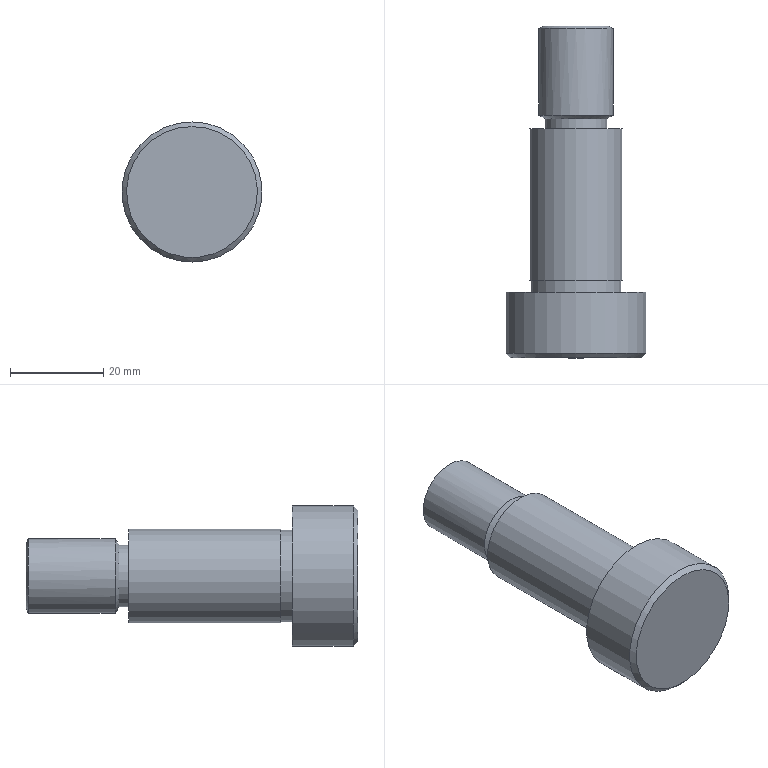Part | STEP file | SCREW-4_id658_x_t | 1 solid | 13 faces | box 30 x 71 x 30 mm | volume 25054 mm3 | plane 5 | cylinder 5 | cone 3 | commonest cylinder face diameters 13.2 x1 16 x1 19.5 x1 20 x1 30 x1
STEP:
#1=CARTESIAN_POINT('',(-162.,76.5,124.));
#2=VERTEX_POINT('',#1);
#3=CARTESIAN_POINT('',(-162.,76.5,110.));
#4=DIRECTION('',(0.,1.,0.));
#5=DIRECTION('',(0.,0.,1.));
#6=AXIS2_PLACEMENT_3D('',#3,#4,#5);
#7=CIRCLE('',#6,14.);
#8=EDGE_CURVE('',#2,#2,#7,.T.);
#9=ORIENTED_EDGE('',*,*,#8,.F.);
#10=EDGE_LOOP('',(#9));
#11=FACE_OUTER_BOUND('',#10,.T.);
#12=CARTESIAN_POINT('',(-162.,76.5,110.));
#13=DIRECTION('',(0.,-1.,0.));
#14=DIRECTION('',(0.,0.,-1.));
#15=AXIS2_PLACEMENT_3D('',#12,#13,#14);
#16=PLANE('',#15);
#17=ADVANCED_FACE('',(#11),#16,.T.);
#18=CARTESIAN_POINT('',(-162.,147.5,103.));
#19=VERTEX_POINT('',#18);
#20=CARTESIAN_POINT('',(-162.,147.5,110.));
#21=DIRECTION('',(0.,-1.,0.));
#22=DIRECTION('',(0.,0.,-1.));
#23=AXIS2_PLACEMENT_3D('',#20,#21,#22);
#24=CIRCLE('',#23,7.);
#25=EDGE_CURVE('',#19,#19,#24,.T.);
#26=ORIENTED_EDGE('',*,*,#25,.F.);
#27=EDGE_LOOP('',(#26));
#28=FACE_OUTER_BOUND('',#27,.T.);
#29=CARTESIAN_POINT('',(-162.,147.5,110.));
#30=DIRECTION('',(0.,-1.,0.));
#31=DIRECTION('',(0.,0.,-1.));
#32=AXIS2_PLACEMENT_3D('',#29,#30,#31);
#33=PLANE('',#32);
#34=ADVANCED_FACE('',(#28),#33,.F.);
#35=ORIENTED_EDGE('',*,*,#8,.T.);
#36=EDGE_LOOP('',(#35));
#37=FACE_BOUND('',#36,.T.);
#38=CARTESIAN_POINT('',(-162.,77.5,95.));
#39=VERTEX_POINT('',#38);
#40=CARTESIAN_POINT('',(-162.,77.5,110.));
#41=DIRECTION('',(0.,1.,0.));
#42=DIRECTION('',(0.,0.,-1.));
#43=AXIS2_PLACEMENT_3D('',#40,#41,#42);
#44=CIRCLE('',#43,15.);
#45=EDGE_CURVE('',#39,#39,#44,.T.);
#46=ORIENTED_EDGE('',*,*,#45,.F.);
#47=EDGE_LOOP('',(#46));
#48=FACE_BOUND('',#47,.T.);
#49=CARTESIAN_POINT('',(-162.,77.5,110.));
#50=DIRECTION('',(0.,1.,0.));
#51=DIRECTION('',(0.,0.,1.));
#52=AXIS2_PLACEMENT_3D('',#49,#50,#51);
#53=CONICAL_SURFACE('',#52,15.,45.);
#54=ADVANCED_FACE('',(#37,#48),#53,.T.);
#55=ORIENTED_EDGE('',*,*,#25,.T.);
#56=EDGE_LOOP('',(#55));
#57=FACE_BOUND('',#56,.T.);
#58=CARTESIAN_POINT('',(-162.,147.,102.));
#59=VERTEX_POINT('',#58);
#60=CARTESIAN_POINT('',(-162.,147.,110.));
#61=DIRECTION('',(0.,-1.,0.));
#62=DIRECTION('',(0.,0.,-1.));
#63=AXIS2_PLACEMENT_3D('',#60,#61,#62);
#64=CIRCLE('',#63,8.);
#65=EDGE_CURVE('',#59,#59,#64,.T.);
#66=ORIENTED_EDGE('',*,*,#65,.F.);
#67=EDGE_LOOP('',(#66));
#68=FACE_BOUND('',#67,.T.);
#69=CARTESIAN_POINT('',(-162.,147.,110.));
#70=DIRECTION('',(0.,-1.,0.));
#71=DIRECTION('',(0.,0.,-1.));
#72=AXIS2_PLACEMENT_3D('',#69,#70,#71);
#73=CONICAL_SURFACE('',#72,8.,63.435);
#74=ADVANCED_FACE('',(#57,#68),#73,.T.);
#75=ORIENTED_EDGE('',*,*,#45,.T.);
#76=EDGE_LOOP('',(#75));
#77=FACE_BOUND('',#76,.T.);
#78=CARTESIAN_POINT('',(-162.,90.5,95.));
#79=VERTEX_POINT('',#78);
#80=CARTESIAN_POINT('',(-162.,90.5,110.));
#81=DIRECTION('',(0.,-1.,0.));
#82=DIRECTION('',(0.,0.,-1.));
#83=AXIS2_PLACEMENT_3D('',#80,#81,#82);
#84=CIRCLE('',#83,15.);
#85=EDGE_CURVE('',#79,#79,#84,.T.);
#86=ORIENTED_EDGE('',*,*,#85,.T.);
#87=EDGE_LOOP('',(#86));
#88=FACE_BOUND('',#87,.T.);
#89=CARTESIAN_POINT('',(-162.,72.95,110.));
#90=DIRECTION('',(0.,-1.,0.));
#91=DIRECTION('',(0.,0.,-1.));
#92=AXIS2_PLACEMENT_3D('',#89,#90,#91);
#93=CYLINDRICAL_SURFACE('',#92,15.);
#94=ADVANCED_FACE('',(#77,#88),#93,.T.);
#95=ORIENTED_EDGE('',*,*,#65,.T.);
#96=EDGE_LOOP('',(#95));
#97=FACE_BOUND('',#96,.T.);
#98=CARTESIAN_POINT('',(-154.,128.45,110.));
#99=VERTEX_POINT('',#98);
#100=CARTESIAN_POINT('',(-162.,128.45,110.));
#101=DIRECTION('',(0.,-1.,0.));
#102=DIRECTION('',(1.,0.,0.));
#103=AXIS2_PLACEMENT_3D('',#100,#101,#102);
#104=CIRCLE('',#103,8.);
#105=EDGE_CURVE('',#99,#99,#104,.T.);
#106=ORIENTED_EDGE('',*,*,#105,.F.);
#107=EDGE_LOOP('',(#106));
#108=FACE_BOUND('',#107,.T.);
#109=CARTESIAN_POINT('',(-162.,72.95,110.));
#110=DIRECTION('',(0.,-1.,0.));
#111=DIRECTION('',(0.,0.,-1.));
#112=AXIS2_PLACEMENT_3D('',#109,#110,#111);
#113=CYLINDRICAL_SURFACE('',#112,8.);
#114=ADVANCED_FACE('',(#97,#108),#113,.T.);
#115=CARTESIAN_POINT('',(-162.,90.5,100.25));
#116=VERTEX_POINT('',#115);
#117=CARTESIAN_POINT('',(-162.,90.5,110.));
#118=DIRECTION('',(0.,1.,0.));
#119=DIRECTION('',(0.,0.,-1.));
#120=AXIS2_PLACEMENT_3D('',#117,#118,#119);
#121=CIRCLE('',#120,9.75);
#122=EDGE_CURVE('',#116,#116,#121,.T.);
#123=ORIENTED_EDGE('',*,*,#122,.F.);
#124=EDGE_LOOP('',(#123));
#125=FACE_BOUND('',#124,.T.);
#126=ORIENTED_EDGE('',*,*,#85,.F.);
#127=EDGE_LOOP('',(#126));
#128=FACE_BOUND('',#127,.T.);
#129=CARTESIAN_POINT('',(-162.,90.5,110.));
#130=DIRECTION('',(0.,-1.,0.));
#131=DIRECTION('',(0.,0.,-1.));
#132=AXIS2_PLACEMENT_3D('',#129,#130,#131);
#133=PLANE('',#132);
#134=ADVANCED_FACE('',(#125,#128),#133,.F.);
#135=ORIENTED_EDGE('',*,*,#105,.T.);
#136=EDGE_LOOP('',(#135));
#137=FACE_BOUND('',#136,.T.);
#138=CARTESIAN_POINT('',(-162.,127.642,103.4));
#139=VERTEX_POINT('',#138);
#140=CARTESIAN_POINT('',(-162.,127.642,110.));
#141=DIRECTION('',(0.,-1.,0.));
#142=DIRECTION('',(0.,0.,-1.));
#143=AXIS2_PLACEMENT_3D('',#140,#141,#142);
#144=CIRCLE('',#143,6.6);
#145=EDGE_CURVE('',#139,#139,#144,.T.);
#146=ORIENTED_EDGE('',*,*,#145,.F.);
#147=EDGE_LOOP('',(#146));
#148=FACE_BOUND('',#147,.T.);
#149=CARTESIAN_POINT('',(-162.,128.45,110.));
#150=DIRECTION('',(0.,1.,0.));
#151=DIRECTION('',(0.,0.,1.));
#152=AXIS2_PLACEMENT_3D('',#149,#150,#151);
#153=CONICAL_SURFACE('',#152,8.,60.);
#154=ADVANCED_FACE('',(#137,#148),#153,.T.);
#155=CARTESIAN_POINT('',(-162.,93.,100.25));
#156=VERTEX_POINT('',#155);
#157=CARTESIAN_POINT('',(-162.,93.,110.));
#158=DIRECTION('',(0.,1.,0.));
#159=DIRECTION('',(0.,0.,-1.));
#160=AXIS2_PLACEMENT_3D('',#157,#158,#159);
#161=CIRCLE('',#160,9.75);
#162=EDGE_CURVE('',#156,#156,#161,.T.);
#163=ORIENTED_EDGE('',*,*,#162,.F.);
#164=EDGE_LOOP('',(#163));
#165=FACE_BOUND('',#164,.T.);
#166=ORIENTED_EDGE('',*,*,#122,.T.);
#167=EDGE_LOOP('',(#166));
#168=FACE_BOUND('',#167,.T.);
#169=CARTESIAN_POINT('',(-162.,72.95,110.));
#170=DIRECTION('',(0.,-1.,0.));
#171=DIRECTION('',(0.,0.,-1.));
#172=AXIS2_PLACEMENT_3D('',#169,#170,#171);
#173=CYLINDRICAL_SURFACE('',#172,9.75);
#174=ADVANCED_FACE('',(#165,#168),#173,.T.);
#175=ORIENTED_EDGE('',*,*,#145,.T.);
#176=EDGE_LOOP('',(#175));
#177=FACE_BOUND('',#176,.T.);
#178=CARTESIAN_POINT('',(-162.,125.5,103.4));
#179=VERTEX_POINT('',#178);
#180=CARTESIAN_POINT('',(-162.,125.5,110.));
#181=DIRECTION('',(0.,1.,0.));
#182=DIRECTION('',(0.,0.,-1.));
#183=AXIS2_PLACEMENT_3D('',#180,#181,#182);
#184=CIRCLE('',#183,6.6);
#185=EDGE_CURVE('',#179,#179,#184,.T.);
#186=ORIENTED_EDGE('',*,*,#185,.T.);
#187=EDGE_LOOP('',(#186));
#188=FACE_BOUND('',#187,.T.);
#189=CARTESIAN_POINT('',(-162.,72.95,110.));
#190=DIRECTION('',(0.,-1.,0.));
#191=DIRECTION('',(0.,0.,-1.));
#192=AXIS2_PLACEMENT_3D('',#189,#190,#191);
#193=CYLINDRICAL_SURFACE('',#192,6.6);
#194=ADVANCED_FACE('',(#177,#188),#193,.T.);
#195=ORIENTED_EDGE('',*,*,#162,.T.);
#196=EDGE_LOOP('',(#195));
#197=FACE_BOUND('',#196,.T.);
#198=CARTESIAN_POINT('',(-162.,93.,100.));
#199=VERTEX_POINT('',#198);
#200=CARTESIAN_POINT('',(-162.,93.,110.));
#201=DIRECTION('',(0.,1.,0.));
#202=DIRECTION('',(0.,0.,-1.));
#203=AXIS2_PLACEMENT_3D('',#200,#201,#202);
#204=CIRCLE('',#203,10.);
#205=EDGE_CURVE('',#199,#199,#204,.T.);
#206=ORIENTED_EDGE('',*,*,#205,.F.);
#207=EDGE_LOOP('',(#206));
#208=FACE_BOUND('',#207,.T.);
#209=CARTESIAN_POINT('',(-162.,93.,110.));
#210=DIRECTION('',(0.,-1.,0.));
#211=DIRECTION('',(0.,0.,-1.));
#212=AXIS2_PLACEMENT_3D('',#209,#210,#211);
#213=PLANE('',#212);
#214=ADVANCED_FACE('',(#197,#208),#213,.T.);
#215=ORIENTED_EDGE('',*,*,#185,.F.);
#216=EDGE_LOOP('',(#215));
#217=FACE_BOUND('',#216,.T.);
#218=CARTESIAN_POINT('',(-162.,125.5,100.));
#219=VERTEX_POINT('',#218);
#220=CARTESIAN_POINT('',(-162.,125.5,110.));
#221=DIRECTION('',(0.,-1.,0.));
#222=DIRECTION('',(0.,0.,-1.));
#223=AXIS2_PLACEMENT_3D('',#220,#221,#222);
#224=CIRCLE('',#223,10.);
#225=EDGE_CURVE('',#219,#219,#224,.T.);
#226=ORIENTED_EDGE('',*,*,#225,.F.);
#227=EDGE_LOOP('',(#226));
#228=FACE_BOUND('',#227,.T.);
#229=CARTESIAN_POINT('',(-162.,125.5,110.));
#230=DIRECTION('',(0.,-1.,0.));
#231=DIRECTION('',(0.,0.,-1.));
#232=AXIS2_PLACEMENT_3D('',#229,#230,#231);
#233=PLANE('',#232);
#234=ADVANCED_FACE('',(#217,#228),#233,.F.);
#235=ORIENTED_EDGE('',*,*,#225,.T.);
#236=EDGE_LOOP('',(#235));
#237=FACE_BOUND('',#236,.T.);
#238=ORIENTED_EDGE('',*,*,#205,.T.);
#239=EDGE_LOOP('',(#238));
#240=FACE_BOUND('',#239,.T.);
#241=CARTESIAN_POINT('',(-162.,72.95,110.));
#242=DIRECTION('',(0.,-1.,0.));
#243=DIRECTION('',(0.,0.,-1.));
#244=AXIS2_PLACEMENT_3D('',#241,#242,#243);
#245=CYLINDRICAL_SURFACE('',#244,10.);
#246=ADVANCED_FACE('',(#237,#240),#245,.T.);
#247=CLOSED_SHELL('',(#17,#34,#54,#74,#94,#114,#134,#154,#174,#194,#214,#234,#246));
#248=MANIFOLD_SOLID_BREP('',#247);
#249=(LENGTH_UNIT()NAMED_UNIT(*)SI_UNIT(.MILLI.,.METRE.));
#250=UNCERTAINTY_MEASURE_WITH_UNIT(LENGTH_MEASURE(0.00002),#249,'','');
#251=(NAMED_UNIT(*)PLANE_ANGLE_UNIT()SI_UNIT($,.RADIAN.));
#252=PLANE_ANGLE_MEASURE_WITH_UNIT(PLANE_ANGLE_MEASURE(0.01745),#251);
#253=DIMENSIONAL_EXPONENTS(0.,0.,0.,0.,0.,0.,0.);
#254=(CONVERSION_BASED_UNIT('DEGREE',#252)NAMED_UNIT(#253)PLANE_ANGLE_UNIT());
#255=(NAMED_UNIT(*)SI_UNIT($,.STERADIAN.)SOLID_ANGLE_UNIT());
#256=(GEOMETRIC_REPRESENTATION_CONTEXT(3)GLOBAL_UNCERTAINTY_ASSIGNED_CONTEXT((#250))GLOBAL_UNIT_ASSIGNED_CONTEXT((#249,#254,#255))REPRESENTATION_CONTEXT('',''));
#257=ADVANCED_BREP_SHAPE_REPRESENTATION('',(#248),#256);